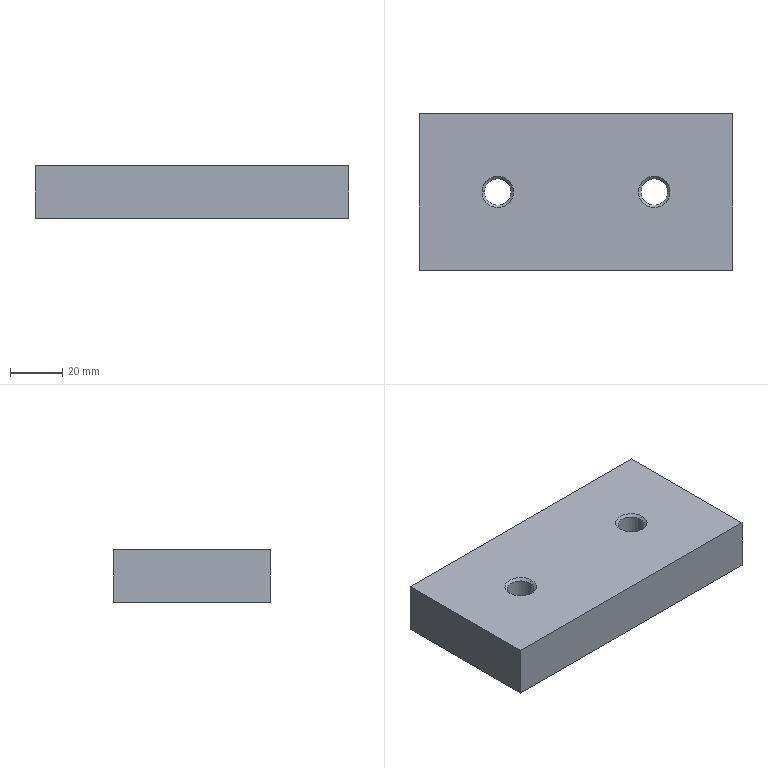Part | STEP file | Street block | 1 solid | 14 faces | box 120 x 60 x 20 mm | volume 140702 mm3 | plane 6 | cone 4 | cylinder 4 | commonest cylinder face diameters 10.2 x4
STEP:
#1=CARTESIAN_POINT('',(0.,0.,0.));
#2=DIRECTION('',(0.,0.,1.));
#3=DIRECTION('',(1.,0.,0.));
#4=AXIS2_PLACEMENT_3D('',#1,#2,#3);
#5=CARTESIAN_POINT('',(-24.9,0.,19.075));
#6=VERTEX_POINT('',#5);
#7=CARTESIAN_POINT('',(-23.975,0.,20.));
#8=VERTEX_POINT('',#7);
#9=CARTESIAN_POINT('',(-23.975,0.,20.));
#10=DIRECTION('',(0.7071,0.,0.7071));
#11=VECTOR('',#10,1.);
#12=LINE('',#9,#11);
#13=CARTESIAN_POINT('',(-30.,0.,20.));
#14=DIRECTION('',(0.,0.,1.));
#15=DIRECTION('',(1.,0.,0.));
#16=AXIS2_PLACEMENT_3D('',#13,#14,#15);
#17=CONICAL_SURFACE('',#16,6.025,0.7854);
#18=CARTESIAN_POINT('',(6.283,0.));
#19=DIRECTION('',(0.,1.));
#20=VECTOR('',#19,1.);
#21=LINE('',#18,#20);
#22=(GEOMETRIC_REPRESENTATION_CONTEXT(2)PARAMETRIC_REPRESENTATION_CONTEXT()REPRESENTATION_CONTEXT('',''));
#23=DEFINITIONAL_REPRESENTATION('',(#21),#22);
#24=PCURVE('',#17,#23);
#25=CARTESIAN_POINT('',(-30.,0.,20.));
#26=DIRECTION('',(0.,0.,1.));
#27=DIRECTION('',(1.,0.,0.));
#28=AXIS2_PLACEMENT_3D('',#25,#26,#27);
#29=CONICAL_SURFACE('',#28,6.025,0.7854);
#30=CARTESIAN_POINT('',(0.,0.));
#31=DIRECTION('',(0.,1.));
#32=VECTOR('',#31,1.);
#33=LINE('',#30,#32);
#34=(GEOMETRIC_REPRESENTATION_CONTEXT(2)PARAMETRIC_REPRESENTATION_CONTEXT()REPRESENTATION_CONTEXT('',''));
#35=DEFINITIONAL_REPRESENTATION('',(#33),#34);
#36=PCURVE('',#29,#35);
#37=SURFACE_CURVE('',#12,(#24,#36),.PCURVE_S1.);
#38=EDGE_CURVE('',#6,#8,#37,.T.);
#39=ORIENTED_EDGE('',*,*,#38,.T.);
#40=CARTESIAN_POINT('',(-36.025,0.,20.));
#41=VERTEX_POINT('',#40);
#42=CARTESIAN_POINT('',(-30.,0.,20.));
#43=DIRECTION('',(0.,0.,1.));
#44=DIRECTION('',(1.,0.,0.));
#45=AXIS2_PLACEMENT_3D('',#42,#43,#44);
#46=CIRCLE('',#45,6.025);
#47=CARTESIAN_POINT('',(0.,0.));
#48=DIRECTION('',(1.,0.));
#49=VECTOR('',#48,1.);
#50=LINE('',#47,#49);
#51=(GEOMETRIC_REPRESENTATION_CONTEXT(2)PARAMETRIC_REPRESENTATION_CONTEXT()REPRESENTATION_CONTEXT('',''));
#52=DEFINITIONAL_REPRESENTATION('',(#50),#51);
#53=PCURVE('',#17,#52);
#54=CARTESIAN_POINT('',(0.,0.,20.));
#55=DIRECTION('',(0.,0.,1.));
#56=DIRECTION('',(1.,0.,0.));
#57=AXIS2_PLACEMENT_3D('',#54,#55,#56);
#58=PLANE('',#57);
#59=CARTESIAN_POINT('',(-30.,0.));
#60=DIRECTION('',(1.,0.));
#61=AXIS2_PLACEMENT_2D('',#59,#60);
#62=CIRCLE('',#61,6.025);
#63=(GEOMETRIC_REPRESENTATION_CONTEXT(2)PARAMETRIC_REPRESENTATION_CONTEXT()REPRESENTATION_CONTEXT('',''));
#64=DEFINITIONAL_REPRESENTATION('',(#62),#63);
#65=PCURVE('',#58,#64);
#66=SURFACE_CURVE('',#46,(#53,#65),.PCURVE_S1.);
#67=EDGE_CURVE('',#41,#8,#66,.T.);
#68=ORIENTED_EDGE('',*,*,#67,.F.);
#69=CARTESIAN_POINT('',(-35.1,0.,19.075));
#70=VERTEX_POINT('',#69);
#71=CARTESIAN_POINT('',(-36.025,0.,20.));
#72=DIRECTION('',(-0.7071,0.,0.7071));
#73=VECTOR('',#72,1.);
#74=LINE('',#71,#73);
#75=CARTESIAN_POINT('',(3.142,0.));
#76=DIRECTION('',(0.,1.));
#77=VECTOR('',#76,1.);
#78=LINE('',#75,#77);
#79=(GEOMETRIC_REPRESENTATION_CONTEXT(2)PARAMETRIC_REPRESENTATION_CONTEXT()REPRESENTATION_CONTEXT('',''));
#80=DEFINITIONAL_REPRESENTATION('',(#78),#79);
#81=PCURVE('',#17,#80);
#82=CARTESIAN_POINT('',(3.142,0.));
#83=DIRECTION('',(0.,1.));
#84=VECTOR('',#83,1.);
#85=LINE('',#82,#84);
#86=(GEOMETRIC_REPRESENTATION_CONTEXT(2)PARAMETRIC_REPRESENTATION_CONTEXT()REPRESENTATION_CONTEXT('',''));
#87=DEFINITIONAL_REPRESENTATION('',(#85),#86);
#88=PCURVE('',#29,#87);
#89=SURFACE_CURVE('',#74,(#81,#88),.PCURVE_S1.);
#90=EDGE_CURVE('',#70,#41,#89,.T.);
#91=ORIENTED_EDGE('',*,*,#90,.F.);
#92=CARTESIAN_POINT('',(-30.,0.,19.075));
#93=DIRECTION('',(0.,0.,1.));
#94=DIRECTION('',(1.,0.,0.));
#95=AXIS2_PLACEMENT_3D('',#92,#93,#94);
#96=CIRCLE('',#95,5.1);
#97=CARTESIAN_POINT('',(0.,-0.925));
#98=DIRECTION('',(1.,0.));
#99=VECTOR('',#98,1.);
#100=LINE('',#97,#99);
#101=(GEOMETRIC_REPRESENTATION_CONTEXT(2)PARAMETRIC_REPRESENTATION_CONTEXT()REPRESENTATION_CONTEXT('',''));
#102=DEFINITIONAL_REPRESENTATION('',(#100),#101);
#103=PCURVE('',#17,#102);
#104=CARTESIAN_POINT('',(-30.,0.,20.));
#105=DIRECTION('',(0.,0.,1.));
#106=DIRECTION('',(1.,0.,0.));
#107=AXIS2_PLACEMENT_3D('',#104,#105,#106);
#108=CYLINDRICAL_SURFACE('',#107,5.1);
#109=CARTESIAN_POINT('',(0.,-0.925));
#110=DIRECTION('',(1.,0.));
#111=VECTOR('',#110,1.);
#112=LINE('',#109,#111);
#113=(GEOMETRIC_REPRESENTATION_CONTEXT(2)PARAMETRIC_REPRESENTATION_CONTEXT()REPRESENTATION_CONTEXT('',''));
#114=DEFINITIONAL_REPRESENTATION('',(#112),#113);
#115=PCURVE('',#108,#114);
#116=SURFACE_CURVE('',#96,(#103,#115),.PCURVE_S1.);
#117=EDGE_CURVE('',#70,#6,#116,.T.);
#118=ORIENTED_EDGE('',*,*,#117,.T.);
#119=EDGE_LOOP('',(#39,#68,#91,#118));
#120=FACE_BOUND('',#119,.F.);
#121=ADVANCED_FACE('',(#120),#17,.F.);
#122=CARTESIAN_POINT('',(-24.9,0.,0.));
#123=VERTEX_POINT('',#122);
#124=CARTESIAN_POINT('',(-24.9,0.,20.));
#125=DIRECTION('',(0.,0.,1.));
#126=VECTOR('',#125,1.);
#127=LINE('',#124,#126);
#128=CARTESIAN_POINT('',(6.283,0.));
#129=DIRECTION('',(0.,1.));
#130=VECTOR('',#129,1.);
#131=LINE('',#128,#130);
#132=(GEOMETRIC_REPRESENTATION_CONTEXT(2)PARAMETRIC_REPRESENTATION_CONTEXT()REPRESENTATION_CONTEXT('',''));
#133=DEFINITIONAL_REPRESENTATION('',(#131),#132);
#134=PCURVE('',#108,#133);
#135=CARTESIAN_POINT('',(-30.,0.,20.));
#136=DIRECTION('',(0.,0.,1.));
#137=DIRECTION('',(1.,0.,0.));
#138=AXIS2_PLACEMENT_3D('',#135,#136,#137);
#139=CYLINDRICAL_SURFACE('',#138,5.1);
#140=CARTESIAN_POINT('',(0.,0.));
#141=DIRECTION('',(0.,1.));
#142=VECTOR('',#141,1.);
#143=LINE('',#140,#142);
#144=(GEOMETRIC_REPRESENTATION_CONTEXT(2)PARAMETRIC_REPRESENTATION_CONTEXT()REPRESENTATION_CONTEXT('',''));
#145=DEFINITIONAL_REPRESENTATION('',(#143),#144);
#146=PCURVE('',#139,#145);
#147=SURFACE_CURVE('',#127,(#134,#146),.PCURVE_S1.);
#148=EDGE_CURVE('',#123,#6,#147,.T.);
#149=ORIENTED_EDGE('',*,*,#148,.T.);
#150=ORIENTED_EDGE('',*,*,#117,.F.);
#151=CARTESIAN_POINT('',(-35.1,0.,0.));
#152=VERTEX_POINT('',#151);
#153=CARTESIAN_POINT('',(-35.1,0.,20.));
#154=DIRECTION('',(0.,0.,1.));
#155=VECTOR('',#154,1.);
#156=LINE('',#153,#155);
#157=CARTESIAN_POINT('',(3.142,0.));
#158=DIRECTION('',(0.,1.));
#159=VECTOR('',#158,1.);
#160=LINE('',#157,#159);
#161=(GEOMETRIC_REPRESENTATION_CONTEXT(2)PARAMETRIC_REPRESENTATION_CONTEXT()REPRESENTATION_CONTEXT('',''));
#162=DEFINITIONAL_REPRESENTATION('',(#160),#161);
#163=PCURVE('',#108,#162);
#164=CARTESIAN_POINT('',(3.142,0.));
#165=DIRECTION('',(0.,1.));
#166=VECTOR('',#165,1.);
#167=LINE('',#164,#166);
#168=(GEOMETRIC_REPRESENTATION_CONTEXT(2)PARAMETRIC_REPRESENTATION_CONTEXT()REPRESENTATION_CONTEXT('',''));
#169=DEFINITIONAL_REPRESENTATION('',(#167),#168);
#170=PCURVE('',#139,#169);
#171=SURFACE_CURVE('',#156,(#163,#170),.PCURVE_S1.);
#172=EDGE_CURVE('',#152,#70,#171,.T.);
#173=ORIENTED_EDGE('',*,*,#172,.F.);
#174=CARTESIAN_POINT('',(-30.,0.,0.));
#175=DIRECTION('',(0.,0.,1.));
#176=DIRECTION('',(1.,0.,0.));
#177=AXIS2_PLACEMENT_3D('',#174,#175,#176);
#178=CIRCLE('',#177,5.1);
#179=CARTESIAN_POINT('',(0.,-20.));
#180=DIRECTION('',(1.,0.));
#181=VECTOR('',#180,1.);
#182=LINE('',#179,#181);
#183=(GEOMETRIC_REPRESENTATION_CONTEXT(2)PARAMETRIC_REPRESENTATION_CONTEXT()REPRESENTATION_CONTEXT('',''));
#184=DEFINITIONAL_REPRESENTATION('',(#182),#183);
#185=PCURVE('',#108,#184);
#186=CARTESIAN_POINT('',(0.,0.,0.));
#187=DIRECTION('',(0.,0.,1.));
#188=DIRECTION('',(1.,0.,0.));
#189=AXIS2_PLACEMENT_3D('',#186,#187,#188);
#190=PLANE('',#189);
#191=CARTESIAN_POINT('',(-30.,0.));
#192=DIRECTION('',(1.,0.));
#193=AXIS2_PLACEMENT_2D('',#191,#192);
#194=CIRCLE('',#193,5.1);
#195=(GEOMETRIC_REPRESENTATION_CONTEXT(2)PARAMETRIC_REPRESENTATION_CONTEXT()REPRESENTATION_CONTEXT('',''));
#196=DEFINITIONAL_REPRESENTATION('',(#194),#195);
#197=PCURVE('',#190,#196);
#198=SURFACE_CURVE('',#178,(#185,#197),.PCURVE_S1.);
#199=EDGE_CURVE('',#152,#123,#198,.T.);
#200=ORIENTED_EDGE('',*,*,#199,.T.);
#201=EDGE_LOOP('',(#149,#150,#173,#200));
#202=FACE_BOUND('',#201,.F.);
#203=ADVANCED_FACE('',(#202),#108,.F.);
#204=CARTESIAN_POINT('',(35.1,0.,19.075));
#205=VERTEX_POINT('',#204);
#206=CARTESIAN_POINT('',(36.025,0.,20.));
#207=VERTEX_POINT('',#206);
#208=CARTESIAN_POINT('',(36.025,0.,20.));
#209=DIRECTION('',(0.7071,0.,0.7071));
#210=VECTOR('',#209,1.);
#211=LINE('',#208,#210);
#212=CARTESIAN_POINT('',(30.,0.,20.));
#213=DIRECTION('',(0.,0.,1.));
#214=DIRECTION('',(1.,0.,0.));
#215=AXIS2_PLACEMENT_3D('',#212,#213,#214);
#216=CONICAL_SURFACE('',#215,6.025,0.7854);
#217=CARTESIAN_POINT('',(6.283,0.));
#218=DIRECTION('',(0.,1.));
#219=VECTOR('',#218,1.);
#220=LINE('',#217,#219);
#221=(GEOMETRIC_REPRESENTATION_CONTEXT(2)PARAMETRIC_REPRESENTATION_CONTEXT()REPRESENTATION_CONTEXT('',''));
#222=DEFINITIONAL_REPRESENTATION('',(#220),#221);
#223=PCURVE('',#216,#222);
#224=CARTESIAN_POINT('',(30.,0.,20.));
#225=DIRECTION('',(0.,0.,1.));
#226=DIRECTION('',(1.,0.,0.));
#227=AXIS2_PLACEMENT_3D('',#224,#225,#226);
#228=CONICAL_SURFACE('',#227,6.025,0.7854);
#229=CARTESIAN_POINT('',(0.,0.));
#230=DIRECTION('',(0.,1.));
#231=VECTOR('',#230,1.);
#232=LINE('',#229,#231);
#233=(GEOMETRIC_REPRESENTATION_CONTEXT(2)PARAMETRIC_REPRESENTATION_CONTEXT()REPRESENTATION_CONTEXT('',''));
#234=DEFINITIONAL_REPRESENTATION('',(#232),#233);
#235=PCURVE('',#228,#234);
#236=SURFACE_CURVE('',#211,(#223,#235),.PCURVE_S1.);
#237=EDGE_CURVE('',#205,#207,#236,.T.);
#238=ORIENTED_EDGE('',*,*,#237,.T.);
#239=CARTESIAN_POINT('',(23.975,0.,20.));
#240=VERTEX_POINT('',#239);
#241=CARTESIAN_POINT('',(30.,0.,20.));
#242=DIRECTION('',(0.,0.,1.));
#243=DIRECTION('',(1.,0.,0.));
#244=AXIS2_PLACEMENT_3D('',#241,#242,#243);
#245=CIRCLE('',#244,6.025);
#246=CARTESIAN_POINT('',(0.,0.));
#247=DIRECTION('',(1.,0.));
#248=VECTOR('',#247,1.);
#249=LINE('',#246,#248);
#250=(GEOMETRIC_REPRESENTATION_CONTEXT(2)PARAMETRIC_REPRESENTATION_CONTEXT()REPRESENTATION_CONTEXT('',''));
#251=DEFINITIONAL_REPRESENTATION('',(#249),#250);
#252=PCURVE('',#216,#251);
#253=CARTESIAN_POINT('',(30.,0.));
#254=DIRECTION('',(1.,0.));
#255=AXIS2_PLACEMENT_2D('',#253,#254);
#256=CIRCLE('',#255,6.025);
#257=(GEOMETRIC_REPRESENTATION_CONTEXT(2)PARAMETRIC_REPRESENTATION_CONTEXT()REPRESENTATION_CONTEXT('',''));
#258=DEFINITIONAL_REPRESENTATION('',(#256),#257);
#259=PCURVE('',#58,#258);
#260=SURFACE_CURVE('',#245,(#252,#259),.PCURVE_S1.);
#261=EDGE_CURVE('',#240,#207,#260,.T.);
#262=ORIENTED_EDGE('',*,*,#261,.F.);
#263=CARTESIAN_POINT('',(24.9,0.,19.075));
#264=VERTEX_POINT('',#263);
#265=CARTESIAN_POINT('',(23.975,0.,20.));
#266=DIRECTION('',(-0.7071,0.,0.7071));
#267=VECTOR('',#266,1.);
#268=LINE('',#265,#267);
#269=CARTESIAN_POINT('',(3.142,0.));
#270=DIRECTION('',(0.,1.));
#271=VECTOR('',#270,1.);
#272=LINE('',#269,#271);
#273=(GEOMETRIC_REPRESENTATION_CONTEXT(2)PARAMETRIC_REPRESENTATION_CONTEXT()REPRESENTATION_CONTEXT('',''));
#274=DEFINITIONAL_REPRESENTATION('',(#272),#273);
#275=PCURVE('',#216,#274);
#276=CARTESIAN_POINT('',(3.142,0.));
#277=DIRECTION('',(0.,1.));
#278=VECTOR('',#277,1.);
#279=LINE('',#276,#278);
#280=(GEOMETRIC_REPRESENTATION_CONTEXT(2)PARAMETRIC_REPRESENTATION_CONTEXT()REPRESENTATION_CONTEXT('',''));
#281=DEFINITIONAL_REPRESENTATION('',(#279),#280);
#282=PCURVE('',#228,#281);
#283=SURFACE_CURVE('',#268,(#275,#282),.PCURVE_S1.);
#284=EDGE_CURVE('',#264,#240,#283,.T.);
#285=ORIENTED_EDGE('',*,*,#284,.F.);
#286=CARTESIAN_POINT('',(30.,0.,19.075));
#287=DIRECTION('',(0.,0.,1.));
#288=DIRECTION('',(1.,0.,0.));
#289=AXIS2_PLACEMENT_3D('',#286,#287,#288);
#290=CIRCLE('',#289,5.1);
#291=CARTESIAN_POINT('',(0.,-0.925));
#292=DIRECTION('',(1.,0.));
#293=VECTOR('',#292,1.);
#294=LINE('',#291,#293);
#295=(GEOMETRIC_REPRESENTATION_CONTEXT(2)PARAMETRIC_REPRESENTATION_CONTEXT()REPRESENTATION_CONTEXT('',''));
#296=DEFINITIONAL_REPRESENTATION('',(#294),#295);
#297=PCURVE('',#216,#296);
#298=CARTESIAN_POINT('',(30.,0.,20.));
#299=DIRECTION('',(0.,0.,1.));
#300=DIRECTION('',(1.,0.,0.));
#301=AXIS2_PLACEMENT_3D('',#298,#299,#300);
#302=CYLINDRICAL_SURFACE('',#301,5.1);
#303=CARTESIAN_POINT('',(0.,-0.925));
#304=DIRECTION('',(1.,0.));
#305=VECTOR('',#304,1.);
#306=LINE('',#303,#305);
#307=(GEOMETRIC_REPRESENTATION_CONTEXT(2)PARAMETRIC_REPRESENTATION_CONTEXT()REPRESENTATION_CONTEXT('',''));
#308=DEFINITIONAL_REPRESENTATION('',(#306),#307);
#309=PCURVE('',#302,#308);
#310=SURFACE_CURVE('',#290,(#297,#309),.PCURVE_S1.);
#311=EDGE_CURVE('',#264,#205,#310,.T.);
#312=ORIENTED_EDGE('',*,*,#311,.T.);
#313=EDGE_LOOP('',(#238,#262,#285,#312));
#314=FACE_BOUND('',#313,.F.);
#315=ADVANCED_FACE('',(#314),#216,.F.);
#316=CARTESIAN_POINT('',(35.1,0.,0.));
#317=VERTEX_POINT('',#316);
#318=CARTESIAN_POINT('',(35.1,0.,20.));
#319=DIRECTION('',(0.,0.,1.));
#320=VECTOR('',#319,1.);
#321=LINE('',#318,#320);
#322=CARTESIAN_POINT('',(6.283,0.));
#323=DIRECTION('',(0.,1.));
#324=VECTOR('',#323,1.);
#325=LINE('',#322,#324);
#326=(GEOMETRIC_REPRESENTATION_CONTEXT(2)PARAMETRIC_REPRESENTATION_CONTEXT()REPRESENTATION_CONTEXT('',''));
#327=DEFINITIONAL_REPRESENTATION('',(#325),#326);
#328=PCURVE('',#302,#327);
#329=CARTESIAN_POINT('',(30.,0.,20.));
#330=DIRECTION('',(0.,0.,1.));
#331=DIRECTION('',(1.,0.,0.));
#332=AXIS2_PLACEMENT_3D('',#329,#330,#331);
#333=CYLINDRICAL_SURFACE('',#332,5.1);
#334=CARTESIAN_POINT('',(0.,0.));
#335=DIRECTION('',(0.,1.));
#336=VECTOR('',#335,1.);
#337=LINE('',#334,#336);
#338=(GEOMETRIC_REPRESENTATION_CONTEXT(2)PARAMETRIC_REPRESENTATION_CONTEXT()REPRESENTATION_CONTEXT('',''));
#339=DEFINITIONAL_REPRESENTATION('',(#337),#338);
#340=PCURVE('',#333,#339);
#341=SURFACE_CURVE('',#321,(#328,#340),.PCURVE_S1.);
#342=EDGE_CURVE('',#317,#205,#341,.T.);
#343=ORIENTED_EDGE('',*,*,#342,.T.);
#344=ORIENTED_EDGE('',*,*,#311,.F.);
#345=CARTESIAN_POINT('',(24.9,0.,0.));
#346=VERTEX_POINT('',#345);
#347=CARTESIAN_POINT('',(24.9,0.,20.));
#348=DIRECTION('',(0.,0.,1.));
#349=VECTOR('',#348,1.);
#350=LINE('',#347,#349);
#351=CARTESIAN_POINT('',(3.142,0.));
#352=DIRECTION('',(0.,1.));
#353=VECTOR('',#352,1.);
#354=LINE('',#351,#353);
#355=(GEOMETRIC_REPRESENTATION_CONTEXT(2)PARAMETRIC_REPRESENTATION_CONTEXT()REPRESENTATION_CONTEXT('',''));
#356=DEFINITIONAL_REPRESENTATION('',(#354),#355);
#357=PCURVE('',#302,#356);
#358=CARTESIAN_POINT('',(3.142,0.));
#359=DIRECTION('',(0.,1.));
#360=VECTOR('',#359,1.);
#361=LINE('',#358,#360);
#362=(GEOMETRIC_REPRESENTATION_CONTEXT(2)PARAMETRIC_REPRESENTATION_CONTEXT()REPRESENTATION_CONTEXT('',''));
#363=DEFINITIONAL_REPRESENTATION('',(#361),#362);
#364=PCURVE('',#333,#363);
#365=SURFACE_CURVE('',#350,(#357,#364),.PCURVE_S1.);
#366=EDGE_CURVE('',#346,#264,#365,.T.);
#367=ORIENTED_EDGE('',*,*,#366,.F.);
#368=CARTESIAN_POINT('',(30.,0.,0.));
#369=DIRECTION('',(0.,0.,1.));
#370=DIRECTION('',(1.,0.,0.));
#371=AXIS2_PLACEMENT_3D('',#368,#369,#370);
#372=CIRCLE('',#371,5.1);
#373=CARTESIAN_POINT('',(0.,-20.));
#374=DIRECTION('',(1.,0.));
#375=VECTOR('',#374,1.);
#376=LINE('',#373,#375);
#377=(GEOMETRIC_REPRESENTATION_CONTEXT(2)PARAMETRIC_REPRESENTATION_CONTEXT()REPRESENTATION_CONTEXT('',''));
#378=DEFINITIONAL_REPRESENTATION('',(#376),#377);
#379=PCURVE('',#302,#378);
#380=CARTESIAN_POINT('',(30.,0.));
#381=DIRECTION('',(1.,0.));
#382=AXIS2_PLACEMENT_2D('',#380,#381);
#383=CIRCLE('',#382,5.1);
#384=(GEOMETRIC_REPRESENTATION_CONTEXT(2)PARAMETRIC_REPRESENTATION_CONTEXT()REPRESENTATION_CONTEXT('',''));
#385=DEFINITIONAL_REPRESENTATION('',(#383),#384);
#386=PCURVE('',#190,#385);
#387=SURFACE_CURVE('',#372,(#379,#386),.PCURVE_S1.);
#388=EDGE_CURVE('',#346,#317,#387,.T.);
#389=ORIENTED_EDGE('',*,*,#388,.T.);
#390=EDGE_LOOP('',(#343,#344,#367,#389));
#391=FACE_BOUND('',#390,.F.);
#392=ADVANCED_FACE('',(#391),#302,.F.);
#393=CARTESIAN_POINT('',(60.,-30.,0.));
#394=VERTEX_POINT('',#393);
#395=CARTESIAN_POINT('',(60.,30.,0.));
#396=VERTEX_POINT('',#395);
#397=CARTESIAN_POINT('',(60.,30.,0.));
#398=DIRECTION('',(0.,1.,0.));
#399=VECTOR('',#398,1.);
#400=LINE('',#397,#399);
#401=CARTESIAN_POINT('',(60.,30.,20.));
#402=DIRECTION('',(-1.,0.,0.));
#403=DIRECTION('',(0.,-1.,0.));
#404=AXIS2_PLACEMENT_3D('',#401,#402,#403);
#405=PLANE('',#404);
#406=CARTESIAN_POINT('',(0.,-20.));
#407=DIRECTION('',(-1.,0.));
#408=VECTOR('',#407,1.);
#409=LINE('',#406,#408);
#410=(GEOMETRIC_REPRESENTATION_CONTEXT(2)PARAMETRIC_REPRESENTATION_CONTEXT()REPRESENTATION_CONTEXT('',''));
#411=DEFINITIONAL_REPRESENTATION('',(#409),#410);
#412=PCURVE('',#405,#411);
#413=CARTESIAN_POINT('',(60.,30.));
#414=DIRECTION('',(0.,1.));
#415=VECTOR('',#414,1.);
#416=LINE('',#413,#415);
#417=(GEOMETRIC_REPRESENTATION_CONTEXT(2)PARAMETRIC_REPRESENTATION_CONTEXT()REPRESENTATION_CONTEXT('',''));
#418=DEFINITIONAL_REPRESENTATION('',(#416),#417);
#419=PCURVE('',#190,#418);
#420=SURFACE_CURVE('',#400,(#412,#419),.PCURVE_S1.);
#421=EDGE_CURVE('',#394,#396,#420,.T.);
#422=ORIENTED_EDGE('',*,*,#421,.T.);
#423=CARTESIAN_POINT('',(60.,30.,20.));
#424=VERTEX_POINT('',#423);
#425=CARTESIAN_POINT('',(60.,30.,20.));
#426=DIRECTION('',(0.,0.,-1.));
#427=VECTOR('',#426,1.);
#428=LINE('',#425,#427);
#429=CARTESIAN_POINT('',(0.,0.));
#430=DIRECTION('',(0.,-1.));
#431=VECTOR('',#430,1.);
#432=LINE('',#429,#431);
#433=(GEOMETRIC_REPRESENTATION_CONTEXT(2)PARAMETRIC_REPRESENTATION_CONTEXT()REPRESENTATION_CONTEXT('',''));
#434=DEFINITIONAL_REPRESENTATION('',(#432),#433);
#435=PCURVE('',#405,#434);
#436=CARTESIAN_POINT('',(-60.,30.,20.));
#437=DIRECTION('',(0.,-1.,0.));
#438=DIRECTION('',(0.,0.,-1.));
#439=AXIS2_PLACEMENT_3D('',#436,#437,#438);
#440=PLANE('',#439);
#441=CARTESIAN_POINT('',(0.,120.));
#442=DIRECTION('',(1.,0.));
#443=VECTOR('',#442,1.);
#444=LINE('',#441,#443);
#445=(GEOMETRIC_REPRESENTATION_CONTEXT(2)PARAMETRIC_REPRESENTATION_CONTEXT()REPRESENTATION_CONTEXT('',''));
#446=DEFINITIONAL_REPRESENTATION('',(#444),#445);
#447=PCURVE('',#440,#446);
#448=SURFACE_CURVE('',#428,(#435,#447),.PCURVE_S1.);
#449=EDGE_CURVE('',#424,#396,#448,.T.);
#450=ORIENTED_EDGE('',*,*,#449,.F.);
#451=CARTESIAN_POINT('',(60.,-30.,20.));
#452=VERTEX_POINT('',#451);
#453=CARTESIAN_POINT('',(60.,30.,20.));
#454=DIRECTION('',(0.,1.,0.));
#455=VECTOR('',#454,1.);
#456=LINE('',#453,#455);
#457=CARTESIAN_POINT('',(0.,0.));
#458=DIRECTION('',(-1.,0.));
#459=VECTOR('',#458,1.);
#460=LINE('',#457,#459);
#461=(GEOMETRIC_REPRESENTATION_CONTEXT(2)PARAMETRIC_REPRESENTATION_CONTEXT()REPRESENTATION_CONTEXT('',''));
#462=DEFINITIONAL_REPRESENTATION('',(#460),#461);
#463=PCURVE('',#405,#462);
#464=CARTESIAN_POINT('',(60.,30.));
#465=DIRECTION('',(0.,1.));
#466=VECTOR('',#465,1.);
#467=LINE('',#464,#466);
#468=(GEOMETRIC_REPRESENTATION_CONTEXT(2)PARAMETRIC_REPRESENTATION_CONTEXT()REPRESENTATION_CONTEXT('',''));
#469=DEFINITIONAL_REPRESENTATION('',(#467),#468);
#470=PCURVE('',#58,#469);
#471=SURFACE_CURVE('',#456,(#463,#470),.PCURVE_S1.);
#472=EDGE_CURVE('',#452,#424,#471,.T.);
#473=ORIENTED_EDGE('',*,*,#472,.F.);
#474=CARTESIAN_POINT('',(60.,-30.,20.));
#475=DIRECTION('',(0.,0.,-1.));
#476=VECTOR('',#475,1.);
#477=LINE('',#474,#476);
#478=CARTESIAN_POINT('',(60.,0.));
#479=DIRECTION('',(0.,-1.));
#480=VECTOR('',#479,1.);
#481=LINE('',#478,#480);
#482=(GEOMETRIC_REPRESENTATION_CONTEXT(2)PARAMETRIC_REPRESENTATION_CONTEXT()REPRESENTATION_CONTEXT('',''));
#483=DEFINITIONAL_REPRESENTATION('',(#481),#482);
#484=PCURVE('',#405,#483);
#485=CARTESIAN_POINT('',(-60.,-30.,20.));
#486=DIRECTION('',(0.,1.,0.));
#487=DIRECTION('',(0.,0.,1.));
#488=AXIS2_PLACEMENT_3D('',#485,#486,#487);
#489=PLANE('',#488);
#490=CARTESIAN_POINT('',(0.,120.));
#491=DIRECTION('',(-1.,0.));
#492=VECTOR('',#491,1.);
#493=LINE('',#490,#492);
#494=(GEOMETRIC_REPRESENTATION_CONTEXT(2)PARAMETRIC_REPRESENTATION_CONTEXT()REPRESENTATION_CONTEXT('',''));
#495=DEFINITIONAL_REPRESENTATION('',(#493),#494);
#496=PCURVE('',#489,#495);
#497=SURFACE_CURVE('',#477,(#484,#496),.PCURVE_S1.);
#498=EDGE_CURVE('',#452,#394,#497,.T.);
#499=ORIENTED_EDGE('',*,*,#498,.T.);
#500=EDGE_LOOP('',(#422,#450,#473,#499));
#501=FACE_BOUND('',#500,.T.);
#502=ADVANCED_FACE('',(#501),#405,.F.);
#503=CARTESIAN_POINT('',(-60.,30.,0.));
#504=VERTEX_POINT('',#503);
#505=CARTESIAN_POINT('',(-60.,30.,0.));
#506=DIRECTION('',(-1.,0.,0.));
#507=VECTOR('',#506,1.);
#508=LINE('',#505,#507);
#509=CARTESIAN_POINT('',(20.,0.));
#510=DIRECTION('',(0.,-1.));
#511=VECTOR('',#510,1.);
#512=LINE('',#509,#511);
#513=(GEOMETRIC_REPRESENTATION_CONTEXT(2)PARAMETRIC_REPRESENTATION_CONTEXT()REPRESENTATION_CONTEXT('',''));
#514=DEFINITIONAL_REPRESENTATION('',(#512),#513);
#515=PCURVE('',#440,#514);
#516=CARTESIAN_POINT('',(-60.,30.));
#517=DIRECTION('',(-1.,0.));
#518=VECTOR('',#517,1.);
#519=LINE('',#516,#518);
#520=(GEOMETRIC_REPRESENTATION_CONTEXT(2)PARAMETRIC_REPRESENTATION_CONTEXT()REPRESENTATION_CONTEXT('',''));
#521=DEFINITIONAL_REPRESENTATION('',(#519),#520);
#522=PCURVE('',#190,#521);
#523=SURFACE_CURVE('',#508,(#515,#522),.PCURVE_S1.);
#524=EDGE_CURVE('',#396,#504,#523,.T.);
#525=ORIENTED_EDGE('',*,*,#524,.T.);
#526=CARTESIAN_POINT('',(-60.,30.,20.));
#527=VERTEX_POINT('',#526);
#528=CARTESIAN_POINT('',(-60.,30.,20.));
#529=DIRECTION('',(0.,0.,-1.));
#530=VECTOR('',#529,1.);
#531=LINE('',#528,#530);
#532=CARTESIAN_POINT('',(0.,0.));
#533=DIRECTION('',(1.,0.));
#534=VECTOR('',#533,1.);
#535=LINE('',#532,#534);
#536=(GEOMETRIC_REPRESENTATION_CONTEXT(2)PARAMETRIC_REPRESENTATION_CONTEXT()REPRESENTATION_CONTEXT('',''));
#537=DEFINITIONAL_REPRESENTATION('',(#535),#536);
#538=PCURVE('',#440,#537);
#539=CARTESIAN_POINT('',(-60.,30.,20.));
#540=DIRECTION('',(1.,0.,0.));
#541=DIRECTION('',(0.,1.,0.));
#542=AXIS2_PLACEMENT_3D('',#539,#540,#541);
#543=PLANE('',#542);
#544=CARTESIAN_POINT('',(0.,0.));
#545=DIRECTION('',(0.,-1.));
#546=VECTOR('',#545,1.);
#547=LINE('',#544,#546);
#548=(GEOMETRIC_REPRESENTATION_CONTEXT(2)PARAMETRIC_REPRESENTATION_CONTEXT()REPRESENTATION_CONTEXT('',''));
#549=DEFINITIONAL_REPRESENTATION('',(#547),#548);
#550=PCURVE('',#543,#549);
#551=SURFACE_CURVE('',#531,(#538,#550),.PCURVE_S1.);
#552=EDGE_CURVE('',#527,#504,#551,.T.);
#553=ORIENTED_EDGE('',*,*,#552,.F.);
#554=CARTESIAN_POINT('',(-60.,30.,20.));
#555=DIRECTION('',(-1.,0.,0.));
#556=VECTOR('',#555,1.);
#557=LINE('',#554,#556);
#558=CARTESIAN_POINT('',(0.,0.));
#559=DIRECTION('',(0.,-1.));
#560=VECTOR('',#559,1.);
#561=LINE('',#558,#560);
#562=(GEOMETRIC_REPRESENTATION_CONTEXT(2)PARAMETRIC_REPRESENTATION_CONTEXT()REPRESENTATION_CONTEXT('',''));
#563=DEFINITIONAL_REPRESENTATION('',(#561),#562);
#564=PCURVE('',#440,#563);
#565=CARTESIAN_POINT('',(-60.,30.));
#566=DIRECTION('',(-1.,0.));
#567=VECTOR('',#566,1.);
#568=LINE('',#565,#567);
#569=(GEOMETRIC_REPRESENTATION_CONTEXT(2)PARAMETRIC_REPRESENTATION_CONTEXT()REPRESENTATION_CONTEXT('',''));
#570=DEFINITIONAL_REPRESENTATION('',(#568),#569);
#571=PCURVE('',#58,#570);
#572=SURFACE_CURVE('',#557,(#564,#571),.PCURVE_S1.);
#573=EDGE_CURVE('',#424,#527,#572,.T.);
#574=ORIENTED_EDGE('',*,*,#573,.F.);
#575=ORIENTED_EDGE('',*,*,#449,.T.);
#576=EDGE_LOOP('',(#525,#553,#574,#575));
#577=FACE_BOUND('',#576,.T.);
#578=ADVANCED_FACE('',(#577),#440,.F.);
#579=CARTESIAN_POINT('',(-60.,-30.,0.));
#580=VERTEX_POINT('',#579);
#581=CARTESIAN_POINT('',(-60.,30.,0.));
#582=DIRECTION('',(0.,-1.,0.));
#583=VECTOR('',#582,1.);
#584=LINE('',#581,#583);
#585=CARTESIAN_POINT('',(0.,-20.));
#586=DIRECTION('',(-1.,0.));
#587=VECTOR('',#586,1.);
#588=LINE('',#585,#587);
#589=(GEOMETRIC_REPRESENTATION_CONTEXT(2)PARAMETRIC_REPRESENTATION_CONTEXT()REPRESENTATION_CONTEXT('',''));
#590=DEFINITIONAL_REPRESENTATION('',(#588),#589);
#591=PCURVE('',#543,#590);
#592=CARTESIAN_POINT('',(-60.,30.));
#593=DIRECTION('',(0.,-1.));
#594=VECTOR('',#593,1.);
#595=LINE('',#592,#594);
#596=(GEOMETRIC_REPRESENTATION_CONTEXT(2)PARAMETRIC_REPRESENTATION_CONTEXT()REPRESENTATION_CONTEXT('',''));
#597=DEFINITIONAL_REPRESENTATION('',(#595),#596);
#598=PCURVE('',#190,#597);
#599=SURFACE_CURVE('',#584,(#591,#598),.PCURVE_S1.);
#600=EDGE_CURVE('',#504,#580,#599,.T.);
#601=ORIENTED_EDGE('',*,*,#600,.T.);
#602=CARTESIAN_POINT('',(-60.,-30.,20.));
#603=VERTEX_POINT('',#602);
#604=CARTESIAN_POINT('',(-60.,-30.,20.));
#605=DIRECTION('',(0.,0.,-1.));
#606=VECTOR('',#605,1.);
#607=LINE('',#604,#606);
#608=CARTESIAN_POINT('',(-60.,0.));
#609=DIRECTION('',(0.,-1.));
#610=VECTOR('',#609,1.);
#611=LINE('',#608,#610);
#612=(GEOMETRIC_REPRESENTATION_CONTEXT(2)PARAMETRIC_REPRESENTATION_CONTEXT()REPRESENTATION_CONTEXT('',''));
#613=DEFINITIONAL_REPRESENTATION('',(#611),#612);
#614=PCURVE('',#543,#613);
#615=CARTESIAN_POINT('',(0.,0.));
#616=DIRECTION('',(-1.,0.));
#617=VECTOR('',#616,1.);
#618=LINE('',#615,#617);
#619=(GEOMETRIC_REPRESENTATION_CONTEXT(2)PARAMETRIC_REPRESENTATION_CONTEXT()REPRESENTATION_CONTEXT('',''));
#620=DEFINITIONAL_REPRESENTATION('',(#618),#619);
#621=PCURVE('',#489,#620);
#622=SURFACE_CURVE('',#607,(#614,#621),.PCURVE_S1.);
#623=EDGE_CURVE('',#603,#580,#622,.T.);
#624=ORIENTED_EDGE('',*,*,#623,.F.);
#625=CARTESIAN_POINT('',(-60.,30.,20.));
#626=DIRECTION('',(0.,-1.,0.));
#627=VECTOR('',#626,1.);
#628=LINE('',#625,#627);
#629=CARTESIAN_POINT('',(0.,0.));
#630=DIRECTION('',(-1.,0.));
#631=VECTOR('',#630,1.);
#632=LINE('',#629,#631);
#633=(GEOMETRIC_REPRESENTATION_CONTEXT(2)PARAMETRIC_REPRESENTATION_CONTEXT()REPRESENTATION_CONTEXT('',''));
#634=DEFINITIONAL_REPRESENTATION('',(#632),#633);
#635=PCURVE('',#543,#634);
#636=CARTESIAN_POINT('',(-60.,30.));
#637=DIRECTION('',(0.,-1.));
#638=VECTOR('',#637,1.);
#639=LINE('',#636,#638);
#640=(GEOMETRIC_REPRESENTATION_CONTEXT(2)PARAMETRIC_REPRESENTATION_CONTEXT()REPRESENTATION_CONTEXT('',''));
#641=DEFINITIONAL_REPRESENTATION('',(#639),#640);
#642=PCURVE('',#58,#641);
#643=SURFACE_CURVE('',#628,(#635,#642),.PCURVE_S1.);
#644=EDGE_CURVE('',#527,#603,#643,.T.);
#645=ORIENTED_EDGE('',*,*,#644,.F.);
#646=ORIENTED_EDGE('',*,*,#552,.T.);
#647=EDGE_LOOP('',(#601,#624,#645,#646));
#648=FACE_BOUND('',#647,.T.);
#649=ADVANCED_FACE('',(#648),#543,.F.);
#650=CARTESIAN_POINT('',(-60.,-30.,0.));
#651=DIRECTION('',(1.,0.,0.));
#652=VECTOR('',#651,1.);
#653=LINE('',#650,#652);
#654=CARTESIAN_POINT('',(-20.,0.));
#655=DIRECTION('',(0.,1.));
#656=VECTOR('',#655,1.);
#657=LINE('',#654,#656);
#658=(GEOMETRIC_REPRESENTATION_CONTEXT(2)PARAMETRIC_REPRESENTATION_CONTEXT()REPRESENTATION_CONTEXT('',''));
#659=DEFINITIONAL_REPRESENTATION('',(#657),#658);
#660=PCURVE('',#489,#659);
#661=CARTESIAN_POINT('',(-60.,-30.));
#662=DIRECTION('',(1.,0.));
#663=VECTOR('',#662,1.);
#664=LINE('',#661,#663);
#665=(GEOMETRIC_REPRESENTATION_CONTEXT(2)PARAMETRIC_REPRESENTATION_CONTEXT()REPRESENTATION_CONTEXT('',''));
#666=DEFINITIONAL_REPRESENTATION('',(#664),#665);
#667=PCURVE('',#190,#666);
#668=SURFACE_CURVE('',#653,(#660,#667),.PCURVE_S1.);
#669=EDGE_CURVE('',#580,#394,#668,.T.);
#670=ORIENTED_EDGE('',*,*,#669,.T.);
#671=ORIENTED_EDGE('',*,*,#498,.F.);
#672=CARTESIAN_POINT('',(-60.,-30.,20.));
#673=DIRECTION('',(1.,0.,0.));
#674=VECTOR('',#673,1.);
#675=LINE('',#672,#674);
#676=CARTESIAN_POINT('',(0.,0.));
#677=DIRECTION('',(0.,1.));
#678=VECTOR('',#677,1.);
#679=LINE('',#676,#678);
#680=(GEOMETRIC_REPRESENTATION_CONTEXT(2)PARAMETRIC_REPRESENTATION_CONTEXT()REPRESENTATION_CONTEXT('',''));
#681=DEFINITIONAL_REPRESENTATION('',(#679),#680);
#682=PCURVE('',#489,#681);
#683=CARTESIAN_POINT('',(-60.,-30.));
#684=DIRECTION('',(1.,0.));
#685=VECTOR('',#684,1.);
#686=LINE('',#683,#685);
#687=(GEOMETRIC_REPRESENTATION_CONTEXT(2)PARAMETRIC_REPRESENTATION_CONTEXT()REPRESENTATION_CONTEXT('',''));
#688=DEFINITIONAL_REPRESENTATION('',(#686),#687);
#689=PCURVE('',#58,#688);
#690=SURFACE_CURVE('',#675,(#682,#689),.PCURVE_S1.);
#691=EDGE_CURVE('',#603,#452,#690,.T.);
#692=ORIENTED_EDGE('',*,*,#691,.F.);
#693=ORIENTED_EDGE('',*,*,#623,.T.);
#694=EDGE_LOOP('',(#670,#671,#692,#693));
#695=FACE_BOUND('',#694,.T.);
#696=ADVANCED_FACE('',(#695),#489,.F.);
#697=CARTESIAN_POINT('',(-30.,0.,20.));
#698=DIRECTION('',(0.,0.,1.));
#699=DIRECTION('',(1.,0.,0.));
#700=AXIS2_PLACEMENT_3D('',#697,#698,#699);
#701=CIRCLE('',#700,6.025);
#702=CARTESIAN_POINT('',(-30.,0.));
#703=DIRECTION('',(1.,0.));
#704=AXIS2_PLACEMENT_2D('',#702,#703);
#705=CIRCLE('',#704,6.025);
#706=(GEOMETRIC_REPRESENTATION_CONTEXT(2)PARAMETRIC_REPRESENTATION_CONTEXT()REPRESENTATION_CONTEXT('',''));
#707=DEFINITIONAL_REPRESENTATION('',(#705),#706);
#708=PCURVE('',#58,#707);
#709=CARTESIAN_POINT('',(0.,0.));
#710=DIRECTION('',(1.,0.));
#711=VECTOR('',#710,1.);
#712=LINE('',#709,#711);
#713=(GEOMETRIC_REPRESENTATION_CONTEXT(2)PARAMETRIC_REPRESENTATION_CONTEXT()REPRESENTATION_CONTEXT('',''));
#714=DEFINITIONAL_REPRESENTATION('',(#712),#713);
#715=PCURVE('',#29,#714);
#716=SURFACE_CURVE('',#701,(#708,#715),.PCURVE_S1.);
#717=EDGE_CURVE('',#8,#41,#716,.T.);
#718=ORIENTED_EDGE('',*,*,#717,.F.);
#719=ORIENTED_EDGE('',*,*,#67,.F.);
#720=EDGE_LOOP('',(#718,#719));
#721=FACE_BOUND('',#720,.T.);
#722=CARTESIAN_POINT('',(30.,0.,20.));
#723=DIRECTION('',(0.,0.,1.));
#724=DIRECTION('',(1.,0.,0.));
#725=AXIS2_PLACEMENT_3D('',#722,#723,#724);
#726=CIRCLE('',#725,6.025);
#727=CARTESIAN_POINT('',(30.,0.));
#728=DIRECTION('',(1.,0.));
#729=AXIS2_PLACEMENT_2D('',#727,#728);
#730=CIRCLE('',#729,6.025);
#731=(GEOMETRIC_REPRESENTATION_CONTEXT(2)PARAMETRIC_REPRESENTATION_CONTEXT()REPRESENTATION_CONTEXT('',''));
#732=DEFINITIONAL_REPRESENTATION('',(#730),#731);
#733=PCURVE('',#58,#732);
#734=CARTESIAN_POINT('',(0.,0.));
#735=DIRECTION('',(1.,0.));
#736=VECTOR('',#735,1.);
#737=LINE('',#734,#736);
#738=(GEOMETRIC_REPRESENTATION_CONTEXT(2)PARAMETRIC_REPRESENTATION_CONTEXT()REPRESENTATION_CONTEXT('',''));
#739=DEFINITIONAL_REPRESENTATION('',(#737),#738);
#740=PCURVE('',#228,#739);
#741=SURFACE_CURVE('',#726,(#733,#740),.PCURVE_S1.);
#742=EDGE_CURVE('',#207,#240,#741,.T.);
#743=ORIENTED_EDGE('',*,*,#742,.F.);
#744=ORIENTED_EDGE('',*,*,#261,.F.);
#745=EDGE_LOOP('',(#743,#744));
#746=FACE_BOUND('',#745,.T.);
#747=ORIENTED_EDGE('',*,*,#472,.T.);
#748=ORIENTED_EDGE('',*,*,#573,.T.);
#749=ORIENTED_EDGE('',*,*,#644,.T.);
#750=ORIENTED_EDGE('',*,*,#691,.T.);
#751=EDGE_LOOP('',(#747,#748,#749,#750));
#752=FACE_BOUND('',#751,.T.);
#753=ADVANCED_FACE('',(#721,#746,#752),#58,.T.);
#754=CARTESIAN_POINT('',(-30.,0.,0.));
#755=DIRECTION('',(0.,0.,1.));
#756=DIRECTION('',(1.,0.,0.));
#757=AXIS2_PLACEMENT_3D('',#754,#755,#756);
#758=CIRCLE('',#757,5.1);
#759=CARTESIAN_POINT('',(-30.,0.));
#760=DIRECTION('',(1.,0.));
#761=AXIS2_PLACEMENT_2D('',#759,#760);
#762=CIRCLE('',#761,5.1);
#763=(GEOMETRIC_REPRESENTATION_CONTEXT(2)PARAMETRIC_REPRESENTATION_CONTEXT()REPRESENTATION_CONTEXT('',''));
#764=DEFINITIONAL_REPRESENTATION('',(#762),#763);
#765=PCURVE('',#190,#764);
#766=CARTESIAN_POINT('',(0.,-20.));
#767=DIRECTION('',(1.,0.));
#768=VECTOR('',#767,1.);
#769=LINE('',#766,#768);
#770=(GEOMETRIC_REPRESENTATION_CONTEXT(2)PARAMETRIC_REPRESENTATION_CONTEXT()REPRESENTATION_CONTEXT('',''));
#771=DEFINITIONAL_REPRESENTATION('',(#769),#770);
#772=PCURVE('',#139,#771);
#773=SURFACE_CURVE('',#758,(#765,#772),.PCURVE_S1.);
#774=EDGE_CURVE('',#123,#152,#773,.T.);
#775=ORIENTED_EDGE('',*,*,#774,.T.);
#776=ORIENTED_EDGE('',*,*,#199,.T.);
#777=EDGE_LOOP('',(#775,#776));
#778=FACE_BOUND('',#777,.T.);
#779=CARTESIAN_POINT('',(30.,0.,0.));
#780=DIRECTION('',(0.,0.,1.));
#781=DIRECTION('',(1.,0.,0.));
#782=AXIS2_PLACEMENT_3D('',#779,#780,#781);
#783=CIRCLE('',#782,5.1);
#784=CARTESIAN_POINT('',(30.,0.));
#785=DIRECTION('',(1.,0.));
#786=AXIS2_PLACEMENT_2D('',#784,#785);
#787=CIRCLE('',#786,5.1);
#788=(GEOMETRIC_REPRESENTATION_CONTEXT(2)PARAMETRIC_REPRESENTATION_CONTEXT()REPRESENTATION_CONTEXT('',''));
#789=DEFINITIONAL_REPRESENTATION('',(#787),#788);
#790=PCURVE('',#190,#789);
#791=CARTESIAN_POINT('',(0.,-20.));
#792=DIRECTION('',(1.,0.));
#793=VECTOR('',#792,1.);
#794=LINE('',#791,#793);
#795=(GEOMETRIC_REPRESENTATION_CONTEXT(2)PARAMETRIC_REPRESENTATION_CONTEXT()REPRESENTATION_CONTEXT('',''));
#796=DEFINITIONAL_REPRESENTATION('',(#794),#795);
#797=PCURVE('',#333,#796);
#798=SURFACE_CURVE('',#783,(#790,#797),.PCURVE_S1.);
#799=EDGE_CURVE('',#317,#346,#798,.T.);
#800=ORIENTED_EDGE('',*,*,#799,.T.);
#801=ORIENTED_EDGE('',*,*,#388,.T.);
#802=EDGE_LOOP('',(#800,#801));
#803=FACE_BOUND('',#802,.T.);
#804=ORIENTED_EDGE('',*,*,#421,.F.);
#805=ORIENTED_EDGE('',*,*,#669,.F.);
#806=ORIENTED_EDGE('',*,*,#600,.F.);
#807=ORIENTED_EDGE('',*,*,#524,.F.);
#808=EDGE_LOOP('',(#804,#805,#806,#807));
#809=FACE_BOUND('',#808,.T.);
#810=ADVANCED_FACE('',(#778,#803,#809),#190,.F.);
#811=CARTESIAN_POINT('',(30.,0.,19.075));
#812=DIRECTION('',(0.,0.,1.));
#813=DIRECTION('',(1.,0.,0.));
#814=AXIS2_PLACEMENT_3D('',#811,#812,#813);
#815=CIRCLE('',#814,5.1);
#816=CARTESIAN_POINT('',(0.,-0.925));
#817=DIRECTION('',(1.,0.));
#818=VECTOR('',#817,1.);
#819=LINE('',#816,#818);
#820=(GEOMETRIC_REPRESENTATION_CONTEXT(2)PARAMETRIC_REPRESENTATION_CONTEXT()REPRESENTATION_CONTEXT('',''));
#821=DEFINITIONAL_REPRESENTATION('',(#819),#820);
#822=PCURVE('',#333,#821);
#823=CARTESIAN_POINT('',(0.,-0.925));
#824=DIRECTION('',(1.,0.));
#825=VECTOR('',#824,1.);
#826=LINE('',#823,#825);
#827=(GEOMETRIC_REPRESENTATION_CONTEXT(2)PARAMETRIC_REPRESENTATION_CONTEXT()REPRESENTATION_CONTEXT('',''));
#828=DEFINITIONAL_REPRESENTATION('',(#826),#827);
#829=PCURVE('',#228,#828);
#830=SURFACE_CURVE('',#815,(#822,#829),.PCURVE_S1.);
#831=EDGE_CURVE('',#205,#264,#830,.T.);
#832=ORIENTED_EDGE('',*,*,#831,.F.);
#833=ORIENTED_EDGE('',*,*,#342,.F.);
#834=ORIENTED_EDGE('',*,*,#799,.T.);
#835=ORIENTED_EDGE('',*,*,#366,.T.);
#836=EDGE_LOOP('',(#832,#833,#834,#835));
#837=FACE_BOUND('',#836,.F.);
#838=ADVANCED_FACE('',(#837),#333,.F.);
#839=ORIENTED_EDGE('',*,*,#742,.F.);
#840=ORIENTED_EDGE('',*,*,#237,.F.);
#841=ORIENTED_EDGE('',*,*,#831,.T.);
#842=ORIENTED_EDGE('',*,*,#284,.T.);
#843=EDGE_LOOP('',(#839,#840,#841,#842));
#844=FACE_BOUND('',#843,.F.);
#845=ADVANCED_FACE('',(#844),#228,.F.);
#846=CARTESIAN_POINT('',(-30.,0.,19.075));
#847=DIRECTION('',(0.,0.,1.));
#848=DIRECTION('',(1.,0.,0.));
#849=AXIS2_PLACEMENT_3D('',#846,#847,#848);
#850=CIRCLE('',#849,5.1);
#851=CARTESIAN_POINT('',(0.,-0.925));
#852=DIRECTION('',(1.,0.));
#853=VECTOR('',#852,1.);
#854=LINE('',#851,#853);
#855=(GEOMETRIC_REPRESENTATION_CONTEXT(2)PARAMETRIC_REPRESENTATION_CONTEXT()REPRESENTATION_CONTEXT('',''));
#856=DEFINITIONAL_REPRESENTATION('',(#854),#855);
#857=PCURVE('',#139,#856);
#858=CARTESIAN_POINT('',(0.,-0.925));
#859=DIRECTION('',(1.,0.));
#860=VECTOR('',#859,1.);
#861=LINE('',#858,#860);
#862=(GEOMETRIC_REPRESENTATION_CONTEXT(2)PARAMETRIC_REPRESENTATION_CONTEXT()REPRESENTATION_CONTEXT('',''));
#863=DEFINITIONAL_REPRESENTATION('',(#861),#862);
#864=PCURVE('',#29,#863);
#865=SURFACE_CURVE('',#850,(#857,#864),.PCURVE_S1.);
#866=EDGE_CURVE('',#6,#70,#865,.T.);
#867=ORIENTED_EDGE('',*,*,#866,.F.);
#868=ORIENTED_EDGE('',*,*,#148,.F.);
#869=ORIENTED_EDGE('',*,*,#774,.T.);
#870=ORIENTED_EDGE('',*,*,#172,.T.);
#871=EDGE_LOOP('',(#867,#868,#869,#870));
#872=FACE_BOUND('',#871,.F.);
#873=ADVANCED_FACE('',(#872),#139,.F.);
#874=ORIENTED_EDGE('',*,*,#717,.F.);
#875=ORIENTED_EDGE('',*,*,#38,.F.);
#876=ORIENTED_EDGE('',*,*,#866,.T.);
#877=ORIENTED_EDGE('',*,*,#90,.T.);
#878=EDGE_LOOP('',(#874,#875,#876,#877));
#879=FACE_BOUND('',#878,.F.);
#880=ADVANCED_FACE('',(#879),#29,.F.);
#881=CLOSED_SHELL('',(#121,#203,#315,#392,#502,#578,#649,#696,#753,#810,#838,#845,#873,#880));
#882=MANIFOLD_SOLID_BREP('',#881);
#883=(LENGTH_UNIT()NAMED_UNIT(*)SI_UNIT(.MILLI.,.METRE.));
#884=UNCERTAINTY_MEASURE_WITH_UNIT(LENGTH_MEASURE(0.0000001),#883,'','');
#885=(NAMED_UNIT(*)PLANE_ANGLE_UNIT()SI_UNIT($,.RADIAN.));
#886=(NAMED_UNIT(*)SI_UNIT($,.STERADIAN.)SOLID_ANGLE_UNIT());
#887=(GEOMETRIC_REPRESENTATION_CONTEXT(3)GLOBAL_UNCERTAINTY_ASSIGNED_CONTEXT((#884))GLOBAL_UNIT_ASSIGNED_CONTEXT((#883,#885,#886))REPRESENTATION_CONTEXT('',''));
#888=ADVANCED_BREP_SHAPE_REPRESENTATION('',(#4,#882),#887);